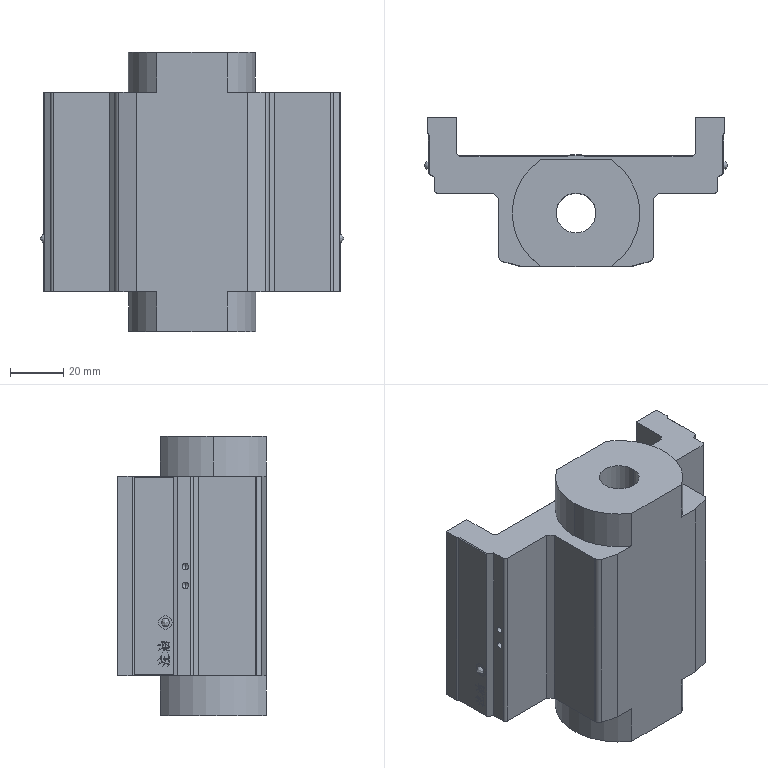Part | SolidWorks | features BaseBody 1 | 1 solid | 217 faces | box 114.08 x 56 x 105 mm | volume 257643 mm3 | plane 111 | cylinder 44 | spline 40 | cone 22 | commonest cylinder face diameters 5 x12 2.5 x8 48 x6 6 x4 15 x4 4 x3